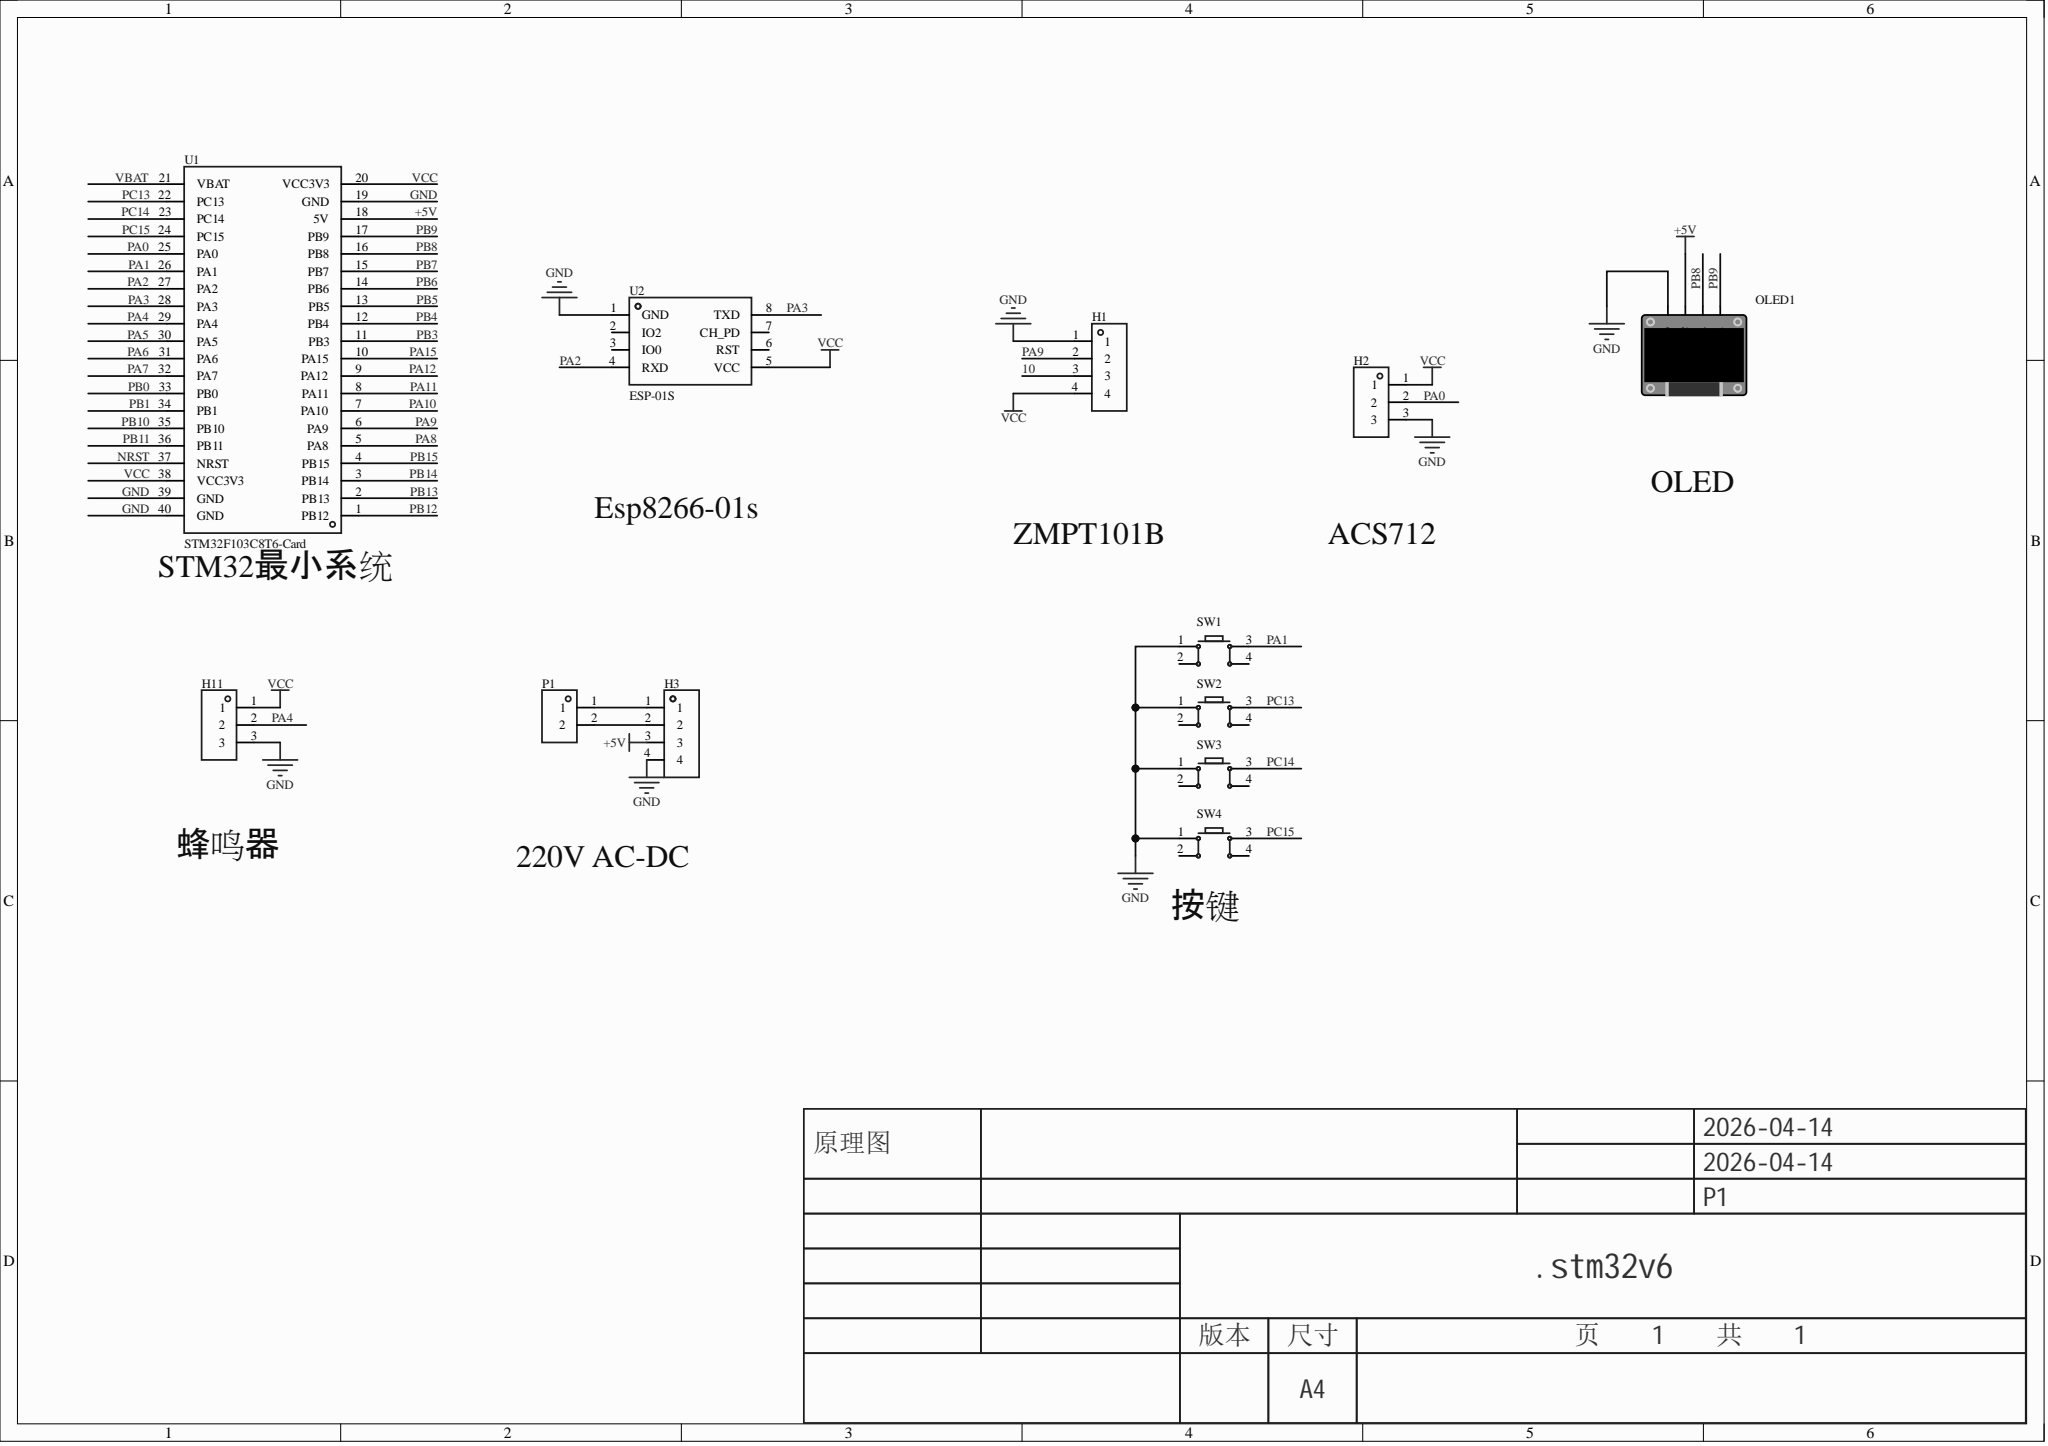Circuit board | Altium Designer | 12 parts | 16 nets
Bill of materials:
Comment,Description,Designator,Footprint,LibRef,Quantity
"","","H1","HDR-TH_4P-P2.54-V-M","HDR-M_2.54_1x4P","1"
"","","H2, H11","HDR-TH_3P-P2.54-V-F","HDR-F_2.54_1x3P","2"
"","","H3","HDR-TH_4P-P2.54-V-F","HDR-F_2.54_1x4P","1"
"","","OLED1","0.96OLED_4P","0.96OLED模块_4P","1"
"KF301-2P接线端子","","P1","CONN-TH_XY301V-A-5.0-2P","KF301-2P接线端子","1"
"","","SW1, SW2, SW3, SW4","SW-TH_4P-L6.0-W6.0-P4.50-LS6.5","Key_TH_6x6x6","4"
"STM32F103C8T6-Card","","U1","CONN-TH_L53.3-W22.9_STM32F103C8T6-CARD","STM32F103C8T6-Card","1"
"ESP-01S","","U2","WIFIM-TH_ESP-01S","ESP-01S_C111009","1"
Netlist (Protel format):
[
H1
HDR-TH_4P-P2.54-V-M




]
[
H2
HDR-TH_3P-P2.54-V-F




]
[
H3
HDR-TH_4P-P2.54-V-F




]
[
H11
HDR-TH_3P-P2.54-V-F




]
[
OLED1
0.96OLED_4P




]
[
P1
CONN-TH_XY301V-A-5.0-2P
KF301-2P接线端子



]
[
SW1
SW-TH_4P-L6.0-W6.0-P4.50-LS6.5




]
[
SW2
SW-TH_4P-L6.0-W6.0-P4.50-LS6.5




]
[
SW3
SW-TH_4P-L6.0-W6.0-P4.50-LS6.5




]
[
SW4
SW-TH_4P-L6.0-W6.0-P4.50-LS6.5




]
[
U1
CONN-TH_L53.3-W22.9_STM32F103C8T6-CARD
STM32F103C8T6-Card



]
[
U2
WIFIM-TH_ESP-01S
ESP-01S



]
(
VCC
H1-4
H2-1
H11-1
U1-20
U1-38
U2-5
)
(
PC15
SW4-3
U1-24
)
(
PC14
SW3-3
U1-23
)
(
PC13
SW2-3
U1-22
)
(
PB9
OLED1-4
U1-17
)
(
PB8
OLED1-3
U1-16
)
(
PA9
H1-2
U1-6
)
(
PA4
H11-2
U1-29
)
(
PA3
U1-28
U2-8
)
(
PA2
U1-27
U2-4
)
(
PA1
SW1-3
U1-26
)
(
PA0
H2-2
U1-25
)
(
NetH3_2
H3-2
P1-2
)
(
NetH3_1
H3-1
P1-1
)
(
GND
H1-1
H2-3
H3-4
H11-3
OLED1-1
SW1-1
SW2-1
SW3-1
SW4-1
U1-19
U1-39
U1-40
U2-1
)
(
+5V
H3-3
OLED1-2
U1-18
)